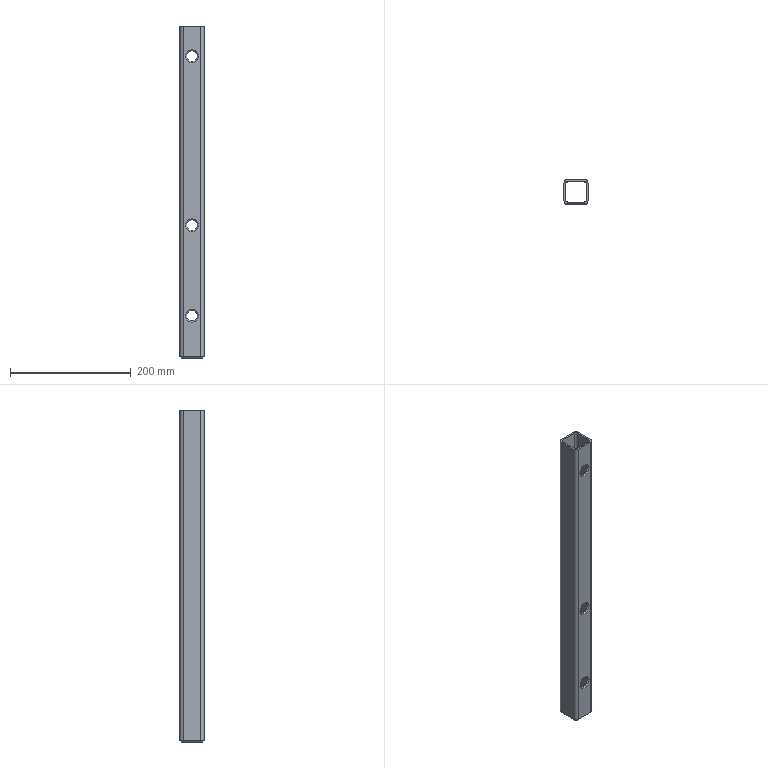Part | STEP file | DIN 59 410 - 40x40x2.9-300 | 1 solid | 38 faces | box 40 x 40 x 550 mm | volume 219599 mm3 | plane 14 | cylinder 14 | cone 10 | commonest cylinder face diameters 17.5 x6 5.8 x4 11.6 x4